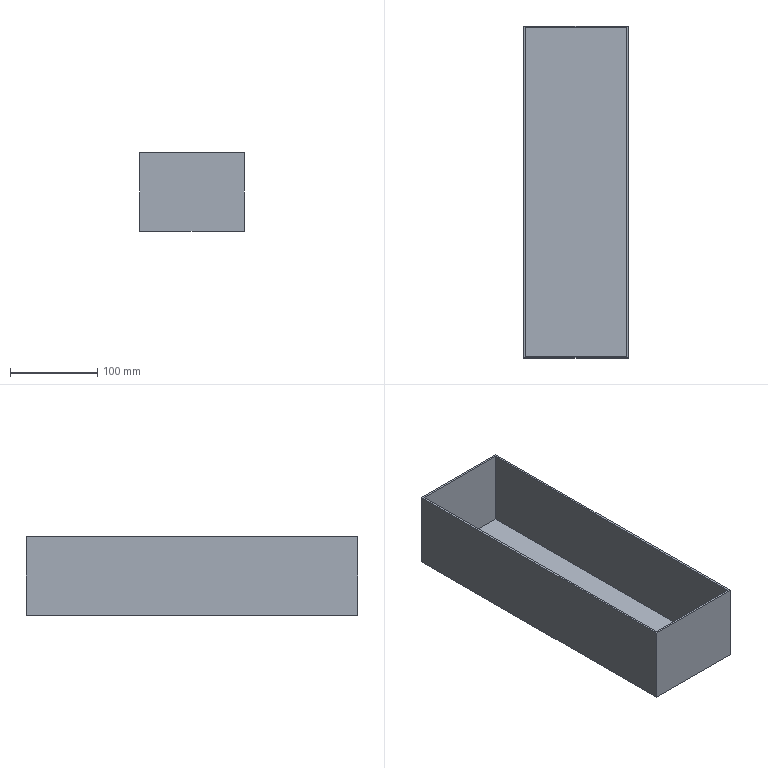Part | NX | features solid 2 | 1 solid | 11 faces | box 120 x 380 x 90 mm | volume 265792 mm3 | plane 11
STEP:
#1=CARTESIAN_POINT('',(-290.,70.,-155.));
#2=VERTEX_POINT('',#1);
#3=CARTESIAN_POINT('',(-410.,70.,-155.));
#4=VERTEX_POINT('',#3);
#5=CARTESIAN_POINT('',(62.831,70.,-155.));
#6=DIRECTION('',(-1.,0.,0.));
#7=VECTOR('',#6,1000.);
#8=LINE('',#5,#7);
#9=EDGE_CURVE('',#2,#4,#8,.T.);
#10=ORIENTED_EDGE('',*,*,#9,.T.);
#11=CARTESIAN_POINT('',(-410.,-310.,-155.));
#12=VERTEX_POINT('',#11);
#13=CARTESIAN_POINT('',(-410.,-840.,-155.));
#14=DIRECTION('',(0.,1.,0.));
#15=VECTOR('',#14,1000.);
#16=LINE('',#13,#15);
#17=EDGE_CURVE('',#12,#4,#16,.T.);
#18=ORIENTED_EDGE('',*,*,#17,.F.);
#19=CARTESIAN_POINT('',(-290.,-310.,-155.));
#20=VERTEX_POINT('',#19);
#21=CARTESIAN_POINT('',(62.831,-310.,-155.));
#22=DIRECTION('',(1.,0.,0.));
#23=VECTOR('',#22,1000.);
#24=LINE('',#21,#23);
#25=EDGE_CURVE('',#20,#12,#24,.F.);
#26=ORIENTED_EDGE('',*,*,#25,.F.);
#27=CARTESIAN_POINT('',(-290.,-840.,-155.));
#28=DIRECTION('',(0.,1.,0.));
#29=VECTOR('',#28,1000.);
#30=LINE('',#27,#29);
#31=EDGE_CURVE('',#20,#2,#30,.T.);
#32=ORIENTED_EDGE('',*,*,#31,.T.);
#33=EDGE_LOOP('',(#10,#18,#26,#32));
#34=FACE_BOUND('',#33,.T.);
#35=CARTESIAN_POINT('',(-292.,68.,-155.));
#36=VERTEX_POINT('',#35);
#37=CARTESIAN_POINT('',(-408.,68.,-155.));
#38=VERTEX_POINT('',#37);
#39=CARTESIAN_POINT('',(62.831,68.,-155.));
#40=DIRECTION('',(-1.,0.,0.));
#41=VECTOR('',#40,1000.);
#42=LINE('',#39,#41);
#43=EDGE_CURVE('',#36,#38,#42,.T.);
#44=ORIENTED_EDGE('',*,*,#43,.F.);
#45=CARTESIAN_POINT('',(-292.,-308.,-155.));
#46=VERTEX_POINT('',#45);
#47=CARTESIAN_POINT('',(-292.,-840.,-155.));
#48=DIRECTION('',(0.,1.,0.));
#49=VECTOR('',#48,1000.);
#50=LINE('',#47,#49);
#51=EDGE_CURVE('',#46,#36,#50,.T.);
#52=ORIENTED_EDGE('',*,*,#51,.F.);
#53=CARTESIAN_POINT('',(-408.,-308.,-155.));
#54=VERTEX_POINT('',#53);
#55=CARTESIAN_POINT('',(62.831,-308.,-155.));
#56=DIRECTION('',(1.,0.,0.));
#57=VECTOR('',#56,1000.);
#58=LINE('',#55,#57);
#59=EDGE_CURVE('',#46,#54,#58,.F.);
#60=ORIENTED_EDGE('',*,*,#59,.T.);
#61=CARTESIAN_POINT('',(-408.,-840.,-155.));
#62=DIRECTION('',(0.,1.,0.));
#63=VECTOR('',#62,1000.);
#64=LINE('',#61,#63);
#65=EDGE_CURVE('',#54,#38,#64,.T.);
#66=ORIENTED_EDGE('',*,*,#65,.T.);
#67=EDGE_LOOP('',(#44,#52,#60,#66));
#68=FACE_BOUND('',#67,.T.);
#69=CARTESIAN_POINT('',(62.831,-840.,-155.));
#70=DIRECTION('',(0.,0.,-1.));
#71=DIRECTION('',(-1.,0.,0.));
#72=AXIS2_PLACEMENT_3D('',#69,#70,#71);
#73=PLANE('',#72);
#74=ADVANCED_FACE('',(#34,#68),#73,.F.);
#75=CARTESIAN_POINT('',(-290.,70.,-245.));
#76=VERTEX_POINT('',#75);
#77=CARTESIAN_POINT('',(-410.,70.,-245.));
#78=VERTEX_POINT('',#77);
#79=CARTESIAN_POINT('',(550.,70.,-245.));
#80=DIRECTION('',(1.,0.,0.));
#81=VECTOR('',#80,1000.);
#82=LINE('',#79,#81);
#83=EDGE_CURVE('',#76,#78,#82,.F.);
#84=ORIENTED_EDGE('',*,*,#83,.F.);
#85=CARTESIAN_POINT('',(-290.,-310.,-245.));
#86=VERTEX_POINT('',#85);
#87=CARTESIAN_POINT('',(-290.,-840.,-245.));
#88=DIRECTION('',(0.,-1.,0.));
#89=VECTOR('',#88,1000.);
#90=LINE('',#87,#89);
#91=EDGE_CURVE('',#86,#76,#90,.F.);
#92=ORIENTED_EDGE('',*,*,#91,.F.);
#93=CARTESIAN_POINT('',(-410.,-310.,-245.));
#94=VERTEX_POINT('',#93);
#95=CARTESIAN_POINT('',(550.,-310.,-245.));
#96=DIRECTION('',(-1.,0.,0.));
#97=VECTOR('',#96,1000.);
#98=LINE('',#95,#97);
#99=EDGE_CURVE('',#86,#94,#98,.T.);
#100=ORIENTED_EDGE('',*,*,#99,.T.);
#101=CARTESIAN_POINT('',(-410.,-840.,-245.));
#102=DIRECTION('',(0.,-1.,0.));
#103=VECTOR('',#102,1000.);
#104=LINE('',#101,#103);
#105=EDGE_CURVE('',#94,#78,#104,.F.);
#106=ORIENTED_EDGE('',*,*,#105,.T.);
#107=EDGE_LOOP('',(#84,#92,#100,#106));
#108=FACE_BOUND('',#107,.T.);
#109=CARTESIAN_POINT('',(550.,-410.,-245.));
#110=DIRECTION('',(0.,0.,1.));
#111=DIRECTION('',(1.,0.,0.));
#112=AXIS2_PLACEMENT_3D('',#109,#110,#111);
#113=PLANE('',#112);
#114=ADVANCED_FACE('',(#108),#113,.F.);
#115=CARTESIAN_POINT('',(-290.,70.,20.));
#116=DIRECTION('',(0.,0.,-1.));
#117=VECTOR('',#116,1000.);
#118=LINE('',#115,#117);
#119=EDGE_CURVE('',#2,#76,#118,.T.);
#120=ORIENTED_EDGE('',*,*,#119,.F.);
#121=ORIENTED_EDGE('',*,*,#31,.F.);
#122=CARTESIAN_POINT('',(-290.,-310.,20.));
#123=DIRECTION('',(0.,0.,1.));
#124=VECTOR('',#123,1000.);
#125=LINE('',#122,#124);
#126=EDGE_CURVE('',#20,#86,#125,.F.);
#127=ORIENTED_EDGE('',*,*,#126,.T.);
#128=ORIENTED_EDGE('',*,*,#91,.T.);
#129=EDGE_LOOP('',(#120,#121,#127,#128));
#130=FACE_BOUND('',#129,.T.);
#131=CARTESIAN_POINT('',(-290.,-840.,20.));
#132=DIRECTION('',(1.,0.,0.));
#133=DIRECTION('',(0.,0.,-1.));
#134=AXIS2_PLACEMENT_3D('',#131,#132,#133);
#135=PLANE('',#134);
#136=ADVANCED_FACE('',(#130),#135,.T.);
#137=CARTESIAN_POINT('',(-410.,70.,20.));
#138=DIRECTION('',(0.,0.,-1.));
#139=VECTOR('',#138,1000.);
#140=LINE('',#137,#139);
#141=EDGE_CURVE('',#4,#78,#140,.T.);
#142=ORIENTED_EDGE('',*,*,#141,.T.);
#143=ORIENTED_EDGE('',*,*,#105,.F.);
#144=CARTESIAN_POINT('',(-410.,-310.,20.));
#145=DIRECTION('',(0.,0.,1.));
#146=VECTOR('',#145,1000.);
#147=LINE('',#144,#146);
#148=EDGE_CURVE('',#12,#94,#147,.F.);
#149=ORIENTED_EDGE('',*,*,#148,.F.);
#150=ORIENTED_EDGE('',*,*,#17,.T.);
#151=EDGE_LOOP('',(#142,#143,#149,#150));
#152=FACE_BOUND('',#151,.T.);
#153=CARTESIAN_POINT('',(-410.,-840.,20.));
#154=DIRECTION('',(1.,0.,0.));
#155=DIRECTION('',(0.,0.,-1.));
#156=AXIS2_PLACEMENT_3D('',#153,#154,#155);
#157=PLANE('',#156);
#158=ADVANCED_FACE('',(#152),#157,.F.);
#159=ORIENTED_EDGE('',*,*,#99,.F.);
#160=ORIENTED_EDGE('',*,*,#126,.F.);
#161=ORIENTED_EDGE('',*,*,#25,.T.);
#162=ORIENTED_EDGE('',*,*,#148,.T.);
#163=EDGE_LOOP('',(#159,#160,#161,#162));
#164=FACE_BOUND('',#163,.T.);
#165=CARTESIAN_POINT('',(590.,-310.,20.));
#166=DIRECTION('',(0.,1.,0.));
#167=DIRECTION('',(-1.,0.,0.));
#168=AXIS2_PLACEMENT_3D('',#165,#166,#167);
#169=PLANE('',#168);
#170=ADVANCED_FACE('',(#164),#169,.F.);
#171=ORIENTED_EDGE('',*,*,#83,.T.);
#172=ORIENTED_EDGE('',*,*,#141,.F.);
#173=ORIENTED_EDGE('',*,*,#9,.F.);
#174=ORIENTED_EDGE('',*,*,#119,.T.);
#175=EDGE_LOOP('',(#171,#172,#173,#174));
#176=FACE_BOUND('',#175,.T.);
#177=CARTESIAN_POINT('',(500.,70.,20.));
#178=DIRECTION('',(0.,-1.,0.));
#179=DIRECTION('',(-1.,0.,0.));
#180=AXIS2_PLACEMENT_3D('',#177,#178,#179);
#181=PLANE('',#180);
#182=ADVANCED_FACE('',(#176),#181,.F.);
#183=CARTESIAN_POINT('',(-292.,68.,-243.));
#184=VERTEX_POINT('',#183);
#185=CARTESIAN_POINT('',(-408.,68.,-243.));
#186=VERTEX_POINT('',#185);
#187=CARTESIAN_POINT('',(550.,68.,-243.));
#188=DIRECTION('',(1.,0.,0.));
#189=VECTOR('',#188,1000.);
#190=LINE('',#187,#189);
#191=EDGE_CURVE('',#184,#186,#190,.F.);
#192=ORIENTED_EDGE('',*,*,#191,.T.);
#193=CARTESIAN_POINT('',(-408.,-308.,-243.));
#194=VERTEX_POINT('',#193);
#195=CARTESIAN_POINT('',(-408.,-840.,-243.));
#196=DIRECTION('',(0.,-1.,0.));
#197=VECTOR('',#196,1000.);
#198=LINE('',#195,#197);
#199=EDGE_CURVE('',#194,#186,#198,.F.);
#200=ORIENTED_EDGE('',*,*,#199,.F.);
#201=CARTESIAN_POINT('',(-292.,-308.,-243.));
#202=VERTEX_POINT('',#201);
#203=CARTESIAN_POINT('',(550.,-308.,-243.));
#204=DIRECTION('',(-1.,0.,0.));
#205=VECTOR('',#204,1000.);
#206=LINE('',#203,#205);
#207=EDGE_CURVE('',#202,#194,#206,.T.);
#208=ORIENTED_EDGE('',*,*,#207,.F.);
#209=CARTESIAN_POINT('',(-292.,-840.,-243.));
#210=DIRECTION('',(0.,-1.,0.));
#211=VECTOR('',#210,1000.);
#212=LINE('',#209,#211);
#213=EDGE_CURVE('',#202,#184,#212,.F.);
#214=ORIENTED_EDGE('',*,*,#213,.T.);
#215=EDGE_LOOP('',(#192,#200,#208,#214));
#216=FACE_BOUND('',#215,.T.);
#217=CARTESIAN_POINT('',(550.,-410.,-243.));
#218=DIRECTION('',(0.,0.,1.));
#219=DIRECTION('',(1.,0.,0.));
#220=AXIS2_PLACEMENT_3D('',#217,#218,#219);
#221=PLANE('',#220);
#222=ADVANCED_FACE('',(#216),#221,.T.);
#223=CARTESIAN_POINT('',(-292.,68.,20.));
#224=DIRECTION('',(0.,0.,-1.));
#225=VECTOR('',#224,1000.);
#226=LINE('',#223,#225);
#227=EDGE_CURVE('',#36,#184,#226,.T.);
#228=ORIENTED_EDGE('',*,*,#227,.T.);
#229=ORIENTED_EDGE('',*,*,#213,.F.);
#230=CARTESIAN_POINT('',(-292.,-308.,20.));
#231=DIRECTION('',(0.,0.,1.));
#232=VECTOR('',#231,1000.);
#233=LINE('',#230,#232);
#234=EDGE_CURVE('',#46,#202,#233,.F.);
#235=ORIENTED_EDGE('',*,*,#234,.F.);
#236=ORIENTED_EDGE('',*,*,#51,.T.);
#237=EDGE_LOOP('',(#228,#229,#235,#236));
#238=FACE_BOUND('',#237,.T.);
#239=CARTESIAN_POINT('',(-292.,-840.,20.));
#240=DIRECTION('',(1.,0.,0.));
#241=DIRECTION('',(0.,0.,-1.));
#242=AXIS2_PLACEMENT_3D('',#239,#240,#241);
#243=PLANE('',#242);
#244=ADVANCED_FACE('',(#238),#243,.F.);
#245=CARTESIAN_POINT('',(-408.,68.,20.));
#246=DIRECTION('',(0.,0.,-1.));
#247=VECTOR('',#246,1000.);
#248=LINE('',#245,#247);
#249=EDGE_CURVE('',#38,#186,#248,.T.);
#250=ORIENTED_EDGE('',*,*,#249,.F.);
#251=ORIENTED_EDGE('',*,*,#65,.F.);
#252=CARTESIAN_POINT('',(-408.,-308.,20.));
#253=DIRECTION('',(0.,0.,1.));
#254=VECTOR('',#253,1000.);
#255=LINE('',#252,#254);
#256=EDGE_CURVE('',#54,#194,#255,.F.);
#257=ORIENTED_EDGE('',*,*,#256,.T.);
#258=ORIENTED_EDGE('',*,*,#199,.T.);
#259=EDGE_LOOP('',(#250,#251,#257,#258));
#260=FACE_BOUND('',#259,.T.);
#261=CARTESIAN_POINT('',(-408.,-840.,20.));
#262=DIRECTION('',(1.,0.,0.));
#263=DIRECTION('',(0.,0.,-1.));
#264=AXIS2_PLACEMENT_3D('',#261,#262,#263);
#265=PLANE('',#264);
#266=ADVANCED_FACE('',(#260),#265,.T.);
#267=ORIENTED_EDGE('',*,*,#207,.T.);
#268=ORIENTED_EDGE('',*,*,#256,.F.);
#269=ORIENTED_EDGE('',*,*,#59,.F.);
#270=ORIENTED_EDGE('',*,*,#234,.T.);
#271=EDGE_LOOP('',(#267,#268,#269,#270));
#272=FACE_BOUND('',#271,.T.);
#273=CARTESIAN_POINT('',(590.,-308.,20.));
#274=DIRECTION('',(0.,1.,0.));
#275=DIRECTION('',(-1.,0.,0.));
#276=AXIS2_PLACEMENT_3D('',#273,#274,#275);
#277=PLANE('',#276);
#278=ADVANCED_FACE('',(#272),#277,.T.);
#279=ORIENTED_EDGE('',*,*,#191,.F.);
#280=ORIENTED_EDGE('',*,*,#227,.F.);
#281=ORIENTED_EDGE('',*,*,#43,.T.);
#282=ORIENTED_EDGE('',*,*,#249,.T.);
#283=EDGE_LOOP('',(#279,#280,#281,#282));
#284=FACE_BOUND('',#283,.T.);
#285=CARTESIAN_POINT('',(500.,68.,20.));
#286=DIRECTION('',(0.,-1.,0.));
#287=DIRECTION('',(-1.,0.,0.));
#288=AXIS2_PLACEMENT_3D('',#285,#286,#287);
#289=PLANE('',#288);
#290=ADVANCED_FACE('',(#284),#289,.T.);
#291=CLOSED_SHELL('',(#74,#114,#136,#158,#170,#182,#222,#244,#266,#278,#290));
#292=MANIFOLD_SOLID_BREP('',#291);
#293=(LENGTH_UNIT()NAMED_UNIT(*)SI_UNIT(.MILLI.,.METRE.));
#294=UNCERTAINTY_MEASURE_WITH_UNIT(LENGTH_MEASURE(0.00001),#293,'','');
#295=(NAMED_UNIT(*)PLANE_ANGLE_UNIT()SI_UNIT($,.RADIAN.));
#296=(NAMED_UNIT(*)SI_UNIT($,.STERADIAN.)SOLID_ANGLE_UNIT());
#297=(GEOMETRIC_REPRESENTATION_CONTEXT(3)GLOBAL_UNCERTAINTY_ASSIGNED_CONTEXT((#294))GLOBAL_UNIT_ASSIGNED_CONTEXT((#293,#295,#296))REPRESENTATION_CONTEXT('',''));
#298=ADVANCED_BREP_SHAPE_REPRESENTATION('',(#292),#297);